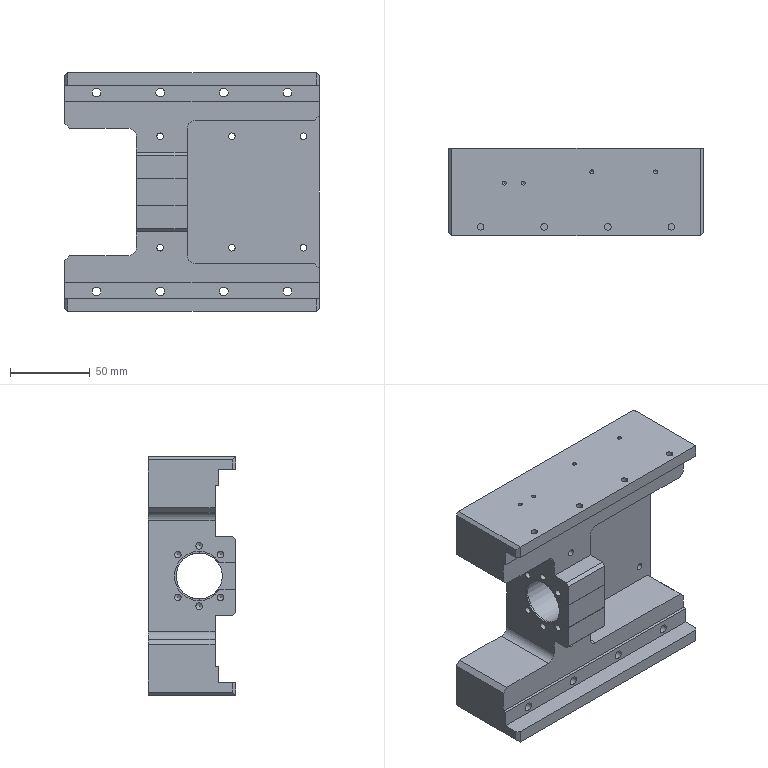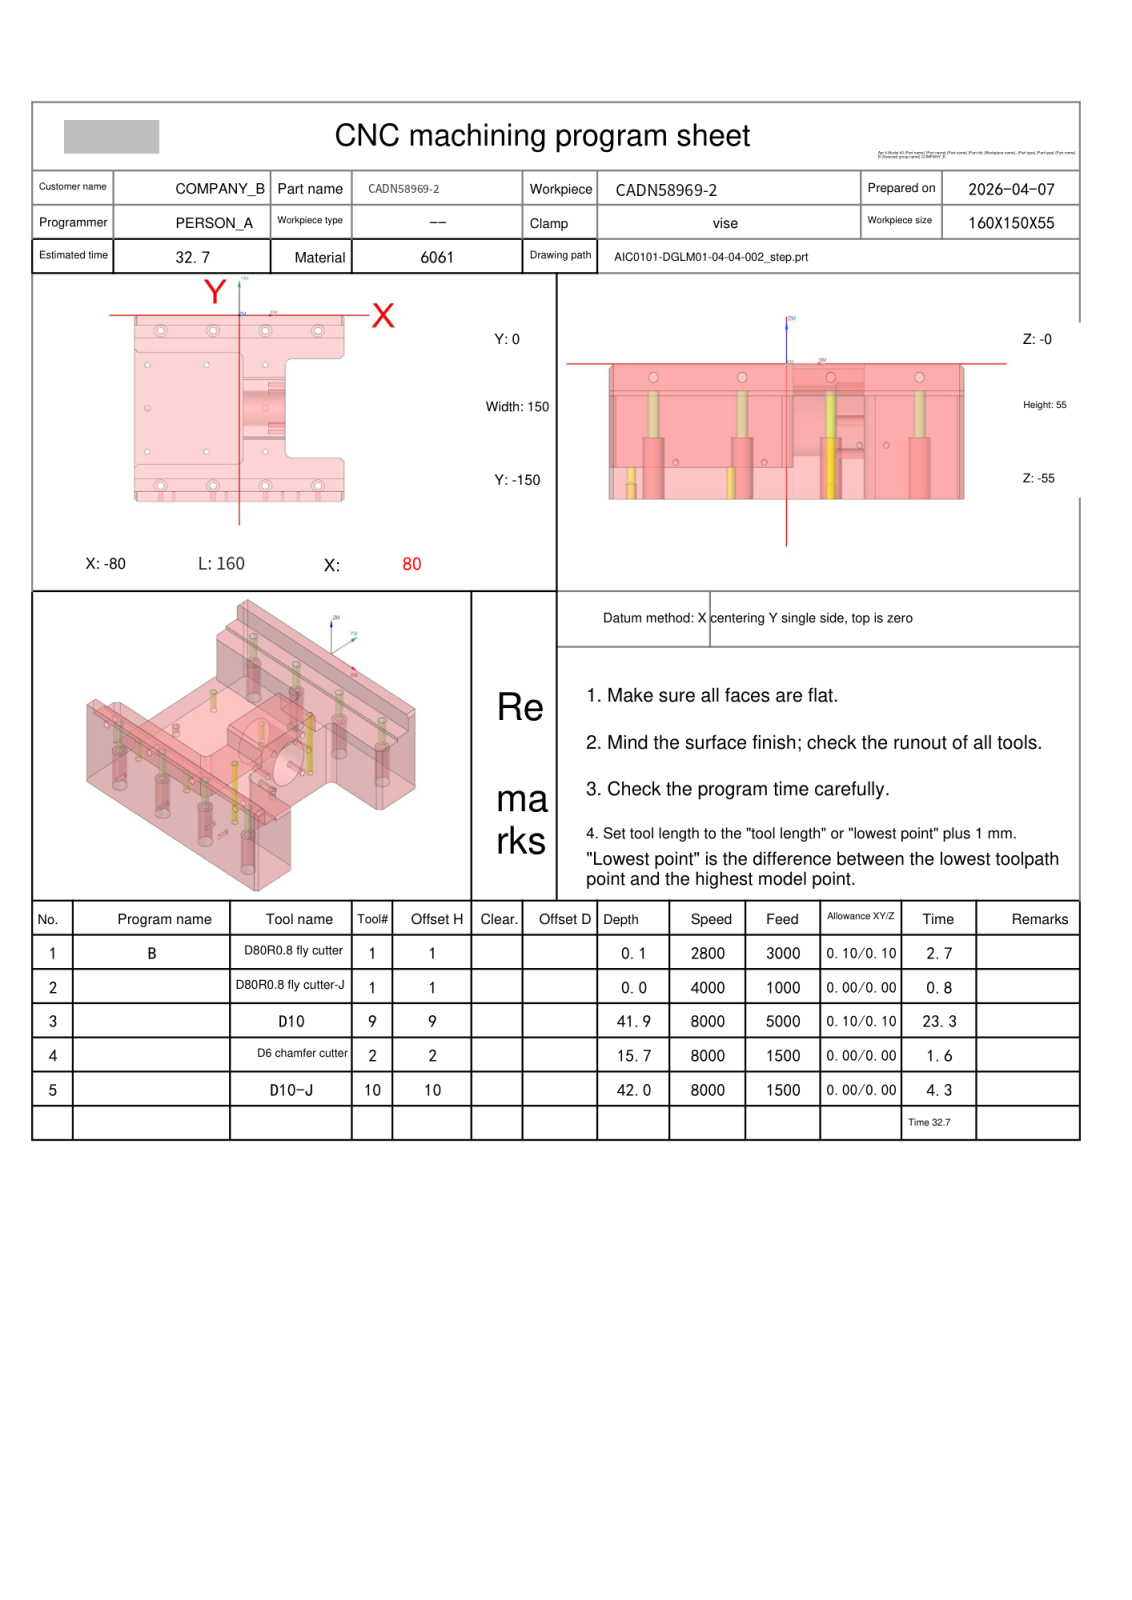NC program | NX | posted by the shop | part box 160 x 55 x 150 mm
Lines 1 to 208 of 14160:
%
O0001
(Machine time: 33.49 MIN)
(===Total Tool:4===)
(T1=D80R0.8 fly cutter D=80. R=0.8 D-H01 Z=-0.   )
(T9=D10     D=10.  R=0.   D-  H09 Z=-41.9 )
(T2=D6 chamfer cutter D=6. R=0. D-H02 Z=-15.7 )
(T10=D10-J  D=10.  R=0.   D10 H10 Z=-42.  )
G80 G90 G17 G49 G40
G91 G28 Z0
M01
N1 T01 M06
(D80R0.8 fly cutter D=80. R=0.8 H=01 ce=0.10 di=0.10)
G00 G90 G54 X-132.097 Y-23.903 M03 S2800
G43 H01 Z20.
M08
Z6.011
G01 Z4.011 F3000.
X-120.097
X112.1
G02 X120.097 Y-31.9 I-.003 J-8.
G01 Y-45.296
G02 X117.755 Y-50.951 I-8. J.001
G01 X99.727 Y-68.979
G02 X94.075 Y-71.32 I-5.655 J5.659
G01 X-112.897
G03 X-120.097 Y-78.52 I0.0 J-7.2
G01 Y-110.737
G03 X-112.097 Y-118.737 I8. J0.0
G01 X120.097
X132.097
Z6.011
G00 X-132.097 Y-23.903
Z5.522
G01 Z3.522
X-120.097
X112.1
G02 X120.097 Y-31.9 I-.003 J-8.
G01 Y-45.296
G02 X117.755 Y-50.951 I-8. J.001
G01 X99.727 Y-68.979
G02 X94.075 Y-71.32 I-5.655 J5.659
G01 X-112.897
G03 X-120.097 Y-78.52 I0.0 J-7.2
G01 Y-110.737
G03 X-112.097 Y-118.737 I8. J0.0
G01 X120.097
X132.097
Z5.522
G00 X-132.097 Y-23.903
Z5.033
G01 Z3.033
X-120.097
X112.1
G02 X120.097 Y-31.9 I-.003 J-8.
G01 Y-45.296
G02 X117.755 Y-50.951 I-8. J.001
G01 X99.727 Y-68.979
G02 X94.075 Y-71.32 I-5.655 J5.659
G01 X-112.897
G03 X-120.097 Y-78.52 I0.0 J-7.2
G01 Y-110.737
G03 X-112.097 Y-118.737 I8. J0.0
G01 X120.097
X132.097
Z5.033
G00 X-132.097 Y-23.903
Z4.544
G01 Z2.544
X-120.097
X112.1
G02 X120.097 Y-31.9 I-.003 J-8.
G01 Y-45.296
G02 X117.755 Y-50.951 I-8. J.001
G01 X99.727 Y-68.979
G02 X94.075 Y-71.32 I-5.655 J5.659
G01 X-112.897
G03 X-120.097 Y-78.52 I0.0 J-7.2
G01 Y-110.737
G03 X-112.097 Y-118.737 I8. J0.0
G01 X120.097
X132.097
Z4.544
G00 Z20.
X-132.097 Y-23.903
Z4.056
G01 Z2.056
X-120.097
X112.1
G02 X120.097 Y-31.9 I-.003 J-8.
G01 Y-45.296
G02 X117.755 Y-50.951 I-8. J.001
G01 X99.727 Y-68.979
G02 X94.075 Y-71.32 I-5.655 J5.659
G01 X-112.897
G03 X-120.097 Y-78.52 I0.0 J-7.2
G01 Y-110.737
G03 X-112.097 Y-118.737 I8. J0.0
G01 X120.097
X132.097
Z4.056
G00 Z20.
X-132.097 Y-23.903
Z3.567
G01 Z1.567
X-120.097
X112.1
G02 X120.097 Y-31.9 I-.003 J-8.
G01 Y-45.296
G02 X117.755 Y-50.951 I-8. J.001
G01 X99.727 Y-68.979
G02 X94.075 Y-71.32 I-5.655 J5.659
G01 X-112.897
G03 X-120.097 Y-78.52 I0.0 J-7.2
G01 Y-110.737
G03 X-112.097 Y-118.737 I8. J0.0
G01 X120.097
X132.097
Z3.567
G00 Z20.
X-132.097 Y-23.903
Z3.078
G01 Z1.078
X-120.097
X112.1
G02 X120.097 Y-31.9 I-.003 J-8.
G01 Y-45.296
G02 X117.755 Y-50.951 I-8. J.001
G01 X99.727 Y-68.979
G02 X94.075 Y-71.32 I-5.655 J5.659
G01 X-112.897
G03 X-120.097 Y-78.52 I0.0 J-7.2
G01 Y-110.737
G03 X-112.097 Y-118.737 I8. J0.0
G01 X120.097
X132.097
Z3.078
G00 Z20.
X-132.097 Y-23.903
Z2.589
G01 Z.589
X-120.097
X112.1
G02 X120.097 Y-31.9 I-.003 J-8.
G01 Y-45.296
G02 X117.755 Y-50.951 I-8. J.001
G01 X99.727 Y-68.979
G02 X94.075 Y-71.32 I-5.655 J5.659
G01 X-112.897
G03 X-120.097 Y-78.52 I0.0 J-7.2
G01 Y-110.737
G03 X-112.097 Y-118.737 I8. J0.0
G01 X120.097
X132.097
Z2.589
G00 Z20.
X-132.097 Y-23.903
Z2.1
G01 Z.1
X-120.097
X112.1
G02 X120.097 Y-31.9 I-.003 J-8.
G01 Y-45.296
G02 X117.755 Y-50.951 I-8. J.001
G01 X99.727 Y-68.979
G02 X94.075 Y-71.32 I-5.655 J5.659
G01 X-112.897
G03 X-120.097 Y-78.52 I0.0 J-7.2
G01 Y-110.737
G03 X-112.097 Y-118.737 I8. J0.0
G01 X120.097
X132.097
Z2.1
G00 Z20.
G91 G28 Z0.0
M05
M09
G91 G28 Z0.0
M01
N2 T01 M06
(D80R0.8 fly cutter-J D=80. R=0.8 H=01 ce=0.00 di=0.00)
G00 G90 G54 X-131.999 Y-24.001 M03 S4000
G43 H01 Z20.
M08
Z2.
G01 Z0.0 F1000.
X-119.999
X112.002
G02 X119.999 Y-31.998 I-.003 J-8.
G01 Y-45.256
G02 X117.657 Y-50.91 I-8. J.001
G01 X99.588 Y-68.979
G02 X93.937 Y-71.32 I-5.655 J5.659
G01 X-112.799
G03 X-119.999 Y-78.52 I0.0 J-7.2
G01 Y-110.639
G03 X-111.999 Y-118.639 I8. J0.0
G01 X119.999
X131.999
Z2.
G00 Z20.
G91 G28 Z0.0
M05
M09
G91 G28 Z0.0
M01